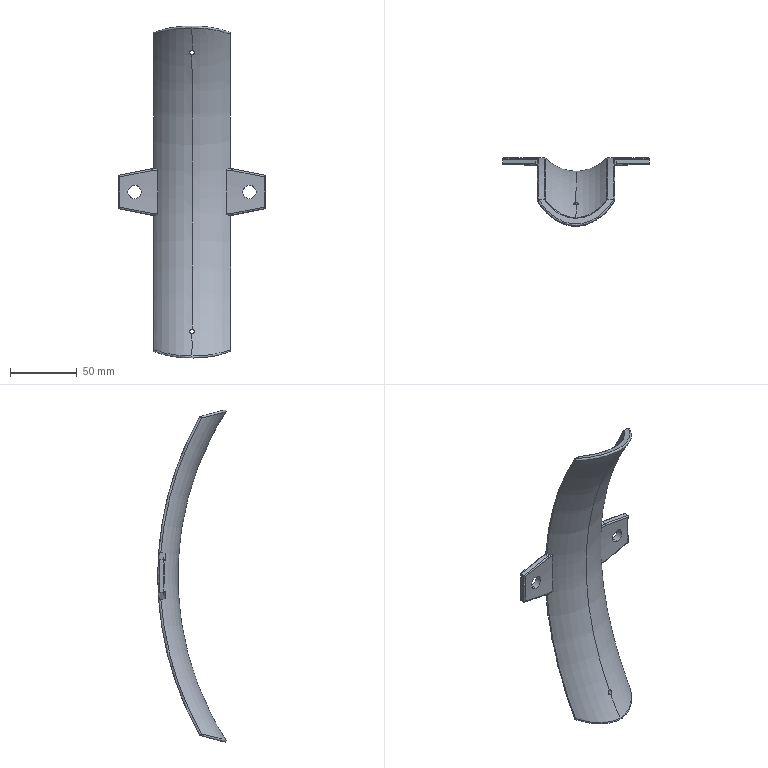Part | SolidWorks | features Chamfer 4, Fillet 2, HoleWzd 2, ICE 2, BossThin 1, Revolution 1, Shell 1 | 1 solid | 70 faces | box 110 x 51.16 x 248.72 mm | volume 85285 mm3 | cylinder 20 | torus 14 | sphere 12 | plane 12 | spline 12 | commonest cylinder face diameters 2 x8 3.3 x4 10 x4 475 x2 485 x2